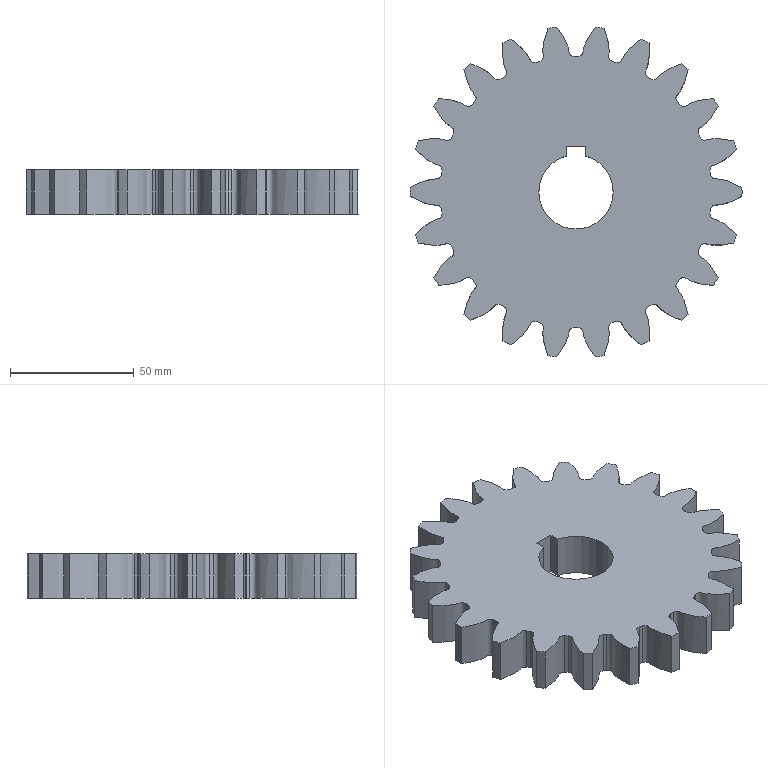Part | SolidWorks | features ICE 2, CirPattern 1, Extrusion 1, RefAxis 1 | 1 solid | 97 faces | box 133.882 x 132.987 x 18 mm | volume 197482 mm3 | cylinder 48 | spline 44 | plane 5 | commonest cylinder face diameters 133.882 x23 109.368 x22 30 x3